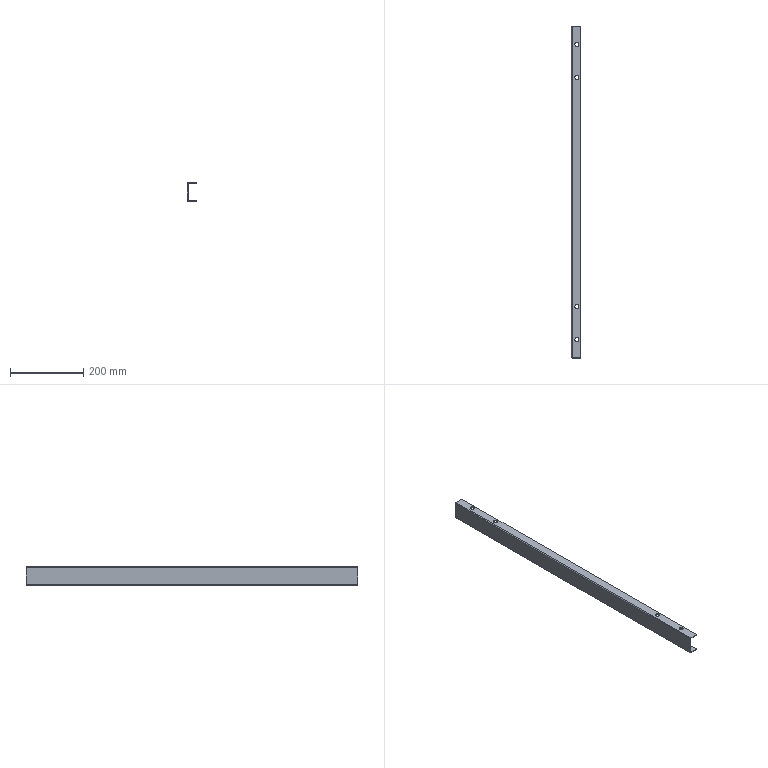Part | SolidWorks | features FlatPattern 1, ICE 1, SMBaseFlange 1, SheetMetal 1 | 1 solid | 38 faces | box 25 x 905 x 50 mm | volume 170375 mm3 | cylinder 20 | plane 18 | commonest cylinder face diameters 11 x16 0.4 x2 4.4 x2
STEP:
#1=CARTESIAN_POINT('',(20.5,402.5,-23.));
#2=VERTEX_POINT('',#1);
#3=CARTESIAN_POINT('',(9.5,402.5,-23.));
#4=VERTEX_POINT('',#3);
#5=CARTESIAN_POINT('',(15.,402.5,-23.));
#6=DIRECTION('',(0.,0.,-1.));
#7=DIRECTION('',(-1.,0.,0.));
#8=AXIS2_PLACEMENT_3D('',#5,#6,#7);
#9=CIRCLE('',#8,5.5);
#10=EDGE_CURVE('',#2,#4,#9,.T.);
#11=ORIENTED_EDGE('',*,*,#10,.F.);
#12=CARTESIAN_POINT('',(20.5,402.5,-25.));
#13=VERTEX_POINT('',#12);
#14=CARTESIAN_POINT('',(20.5,402.5,25.));
#15=DIRECTION('',(0.,0.,-1.));
#16=VECTOR('',#15,1000.);
#17=LINE('',#14,#16);
#18=EDGE_CURVE('',#2,#13,#17,.T.);
#19=ORIENTED_EDGE('',*,*,#18,.T.);
#20=CARTESIAN_POINT('',(9.5,402.5,-25.));
#21=VERTEX_POINT('',#20);
#22=CARTESIAN_POINT('',(15.,402.5,-25.));
#23=DIRECTION('',(0.,0.,-1.));
#24=DIRECTION('',(-1.,0.,0.));
#25=AXIS2_PLACEMENT_3D('',#22,#23,#24);
#26=CIRCLE('',#25,5.5);
#27=EDGE_CURVE('',#13,#21,#26,.T.);
#28=ORIENTED_EDGE('',*,*,#27,.T.);
#29=CARTESIAN_POINT('',(9.5,402.5,25.));
#30=DIRECTION('',(0.,0.,-1.));
#31=VECTOR('',#30,1000.);
#32=LINE('',#29,#31);
#33=EDGE_CURVE('',#4,#21,#32,.T.);
#34=ORIENTED_EDGE('',*,*,#33,.F.);
#35=EDGE_LOOP('',(#11,#19,#28,#34));
#36=FACE_OUTER_BOUND('',#35,.T.);
#37=CARTESIAN_POINT('',(15.,402.5,25.));
#38=DIRECTION('',(0.,0.,-1.));
#39=DIRECTION('',(-1.,0.,0.));
#40=AXIS2_PLACEMENT_3D('',#37,#38,#39);
#41=CYLINDRICAL_SURFACE('',#40,5.5);
#42=ADVANCED_FACE('',(#36),#41,.F.);
#43=CARTESIAN_POINT('',(20.5,312.5,-23.));
#44=VERTEX_POINT('',#43);
#45=CARTESIAN_POINT('',(9.5,312.5,-23.));
#46=VERTEX_POINT('',#45);
#47=CARTESIAN_POINT('',(15.,312.5,-23.));
#48=DIRECTION('',(0.,0.,-1.));
#49=DIRECTION('',(-1.,0.,0.));
#50=AXIS2_PLACEMENT_3D('',#47,#48,#49);
#51=CIRCLE('',#50,5.5);
#52=EDGE_CURVE('',#44,#46,#51,.T.);
#53=ORIENTED_EDGE('',*,*,#52,.F.);
#54=CARTESIAN_POINT('',(20.5,312.5,-25.));
#55=VERTEX_POINT('',#54);
#56=CARTESIAN_POINT('',(20.5,312.5,25.));
#57=DIRECTION('',(0.,0.,-1.));
#58=VECTOR('',#57,1000.);
#59=LINE('',#56,#58);
#60=EDGE_CURVE('',#44,#55,#59,.T.);
#61=ORIENTED_EDGE('',*,*,#60,.T.);
#62=CARTESIAN_POINT('',(9.5,312.5,-25.));
#63=VERTEX_POINT('',#62);
#64=CARTESIAN_POINT('',(15.,312.5,-25.));
#65=DIRECTION('',(0.,0.,-1.));
#66=DIRECTION('',(-1.,0.,0.));
#67=AXIS2_PLACEMENT_3D('',#64,#65,#66);
#68=CIRCLE('',#67,5.5);
#69=EDGE_CURVE('',#55,#63,#68,.T.);
#70=ORIENTED_EDGE('',*,*,#69,.T.);
#71=CARTESIAN_POINT('',(9.5,312.5,25.));
#72=DIRECTION('',(0.,0.,-1.));
#73=VECTOR('',#72,1000.);
#74=LINE('',#71,#73);
#75=EDGE_CURVE('',#46,#63,#74,.T.);
#76=ORIENTED_EDGE('',*,*,#75,.F.);
#77=EDGE_LOOP('',(#53,#61,#70,#76));
#78=FACE_OUTER_BOUND('',#77,.T.);
#79=CARTESIAN_POINT('',(15.,312.5,25.));
#80=DIRECTION('',(0.,0.,-1.));
#81=DIRECTION('',(-1.,0.,0.));
#82=AXIS2_PLACEMENT_3D('',#79,#80,#81);
#83=CYLINDRICAL_SURFACE('',#82,5.5);
#84=ADVANCED_FACE('',(#78),#83,.F.);
#85=CARTESIAN_POINT('',(20.5,-312.5,-23.));
#86=VERTEX_POINT('',#85);
#87=CARTESIAN_POINT('',(9.5,-312.5,-23.));
#88=VERTEX_POINT('',#87);
#89=CARTESIAN_POINT('',(15.,-312.5,-23.));
#90=DIRECTION('',(0.,0.,-1.));
#91=DIRECTION('',(-1.,0.,0.));
#92=AXIS2_PLACEMENT_3D('',#89,#90,#91);
#93=CIRCLE('',#92,5.5);
#94=EDGE_CURVE('',#86,#88,#93,.T.);
#95=ORIENTED_EDGE('',*,*,#94,.F.);
#96=CARTESIAN_POINT('',(20.5,-312.5,-25.));
#97=VERTEX_POINT('',#96);
#98=CARTESIAN_POINT('',(20.5,-312.5,25.));
#99=DIRECTION('',(0.,0.,-1.));
#100=VECTOR('',#99,1000.);
#101=LINE('',#98,#100);
#102=EDGE_CURVE('',#86,#97,#101,.T.);
#103=ORIENTED_EDGE('',*,*,#102,.T.);
#104=CARTESIAN_POINT('',(9.5,-312.5,-25.));
#105=VERTEX_POINT('',#104);
#106=CARTESIAN_POINT('',(15.,-312.5,-25.));
#107=DIRECTION('',(0.,0.,-1.));
#108=DIRECTION('',(-1.,0.,0.));
#109=AXIS2_PLACEMENT_3D('',#106,#107,#108);
#110=CIRCLE('',#109,5.5);
#111=EDGE_CURVE('',#97,#105,#110,.T.);
#112=ORIENTED_EDGE('',*,*,#111,.T.);
#113=CARTESIAN_POINT('',(9.5,-312.5,25.));
#114=DIRECTION('',(0.,0.,-1.));
#115=VECTOR('',#114,1000.);
#116=LINE('',#113,#115);
#117=EDGE_CURVE('',#88,#105,#116,.T.);
#118=ORIENTED_EDGE('',*,*,#117,.F.);
#119=EDGE_LOOP('',(#95,#103,#112,#118));
#120=FACE_OUTER_BOUND('',#119,.T.);
#121=CARTESIAN_POINT('',(15.,-312.5,25.));
#122=DIRECTION('',(0.,0.,-1.));
#123=DIRECTION('',(-1.,0.,0.));
#124=AXIS2_PLACEMENT_3D('',#121,#122,#123);
#125=CYLINDRICAL_SURFACE('',#124,5.5);
#126=ADVANCED_FACE('',(#120),#125,.F.);
#127=CARTESIAN_POINT('',(20.5,-402.5,-23.));
#128=VERTEX_POINT('',#127);
#129=CARTESIAN_POINT('',(9.5,-402.5,-23.));
#130=VERTEX_POINT('',#129);
#131=CARTESIAN_POINT('',(15.,-402.5,-23.));
#132=DIRECTION('',(0.,0.,-1.));
#133=DIRECTION('',(-1.,0.,0.));
#134=AXIS2_PLACEMENT_3D('',#131,#132,#133);
#135=CIRCLE('',#134,5.5);
#136=EDGE_CURVE('',#128,#130,#135,.T.);
#137=ORIENTED_EDGE('',*,*,#136,.F.);
#138=CARTESIAN_POINT('',(20.5,-402.5,-25.));
#139=VERTEX_POINT('',#138);
#140=CARTESIAN_POINT('',(20.5,-402.5,25.));
#141=DIRECTION('',(0.,0.,-1.));
#142=VECTOR('',#141,1000.);
#143=LINE('',#140,#142);
#144=EDGE_CURVE('',#128,#139,#143,.T.);
#145=ORIENTED_EDGE('',*,*,#144,.T.);
#146=CARTESIAN_POINT('',(9.5,-402.5,-25.));
#147=VERTEX_POINT('',#146);
#148=CARTESIAN_POINT('',(15.,-402.5,-25.));
#149=DIRECTION('',(0.,0.,-1.));
#150=DIRECTION('',(-1.,0.,0.));
#151=AXIS2_PLACEMENT_3D('',#148,#149,#150);
#152=CIRCLE('',#151,5.5);
#153=EDGE_CURVE('',#139,#147,#152,.T.);
#154=ORIENTED_EDGE('',*,*,#153,.T.);
#155=CARTESIAN_POINT('',(9.5,-402.5,25.));
#156=DIRECTION('',(0.,0.,-1.));
#157=VECTOR('',#156,1000.);
#158=LINE('',#155,#157);
#159=EDGE_CURVE('',#130,#147,#158,.T.);
#160=ORIENTED_EDGE('',*,*,#159,.F.);
#161=EDGE_LOOP('',(#137,#145,#154,#160));
#162=FACE_OUTER_BOUND('',#161,.T.);
#163=CARTESIAN_POINT('',(15.,-402.5,25.));
#164=DIRECTION('',(0.,0.,-1.));
#165=DIRECTION('',(-1.,0.,0.));
#166=AXIS2_PLACEMENT_3D('',#163,#164,#165);
#167=CYLINDRICAL_SURFACE('',#166,5.5);
#168=ADVANCED_FACE('',(#162),#167,.F.);
#169=CARTESIAN_POINT('',(20.5,402.5,25.));
#170=VERTEX_POINT('',#169);
#171=CARTESIAN_POINT('',(9.5,402.5,25.));
#172=VERTEX_POINT('',#171);
#173=CARTESIAN_POINT('',(15.,402.5,25.));
#174=DIRECTION('',(0.,0.,-1.));
#175=DIRECTION('',(-1.,0.,0.));
#176=AXIS2_PLACEMENT_3D('',#173,#174,#175);
#177=CIRCLE('',#176,5.5);
#178=EDGE_CURVE('',#170,#172,#177,.T.);
#179=ORIENTED_EDGE('',*,*,#178,.F.);
#180=CARTESIAN_POINT('',(20.5,402.5,23.));
#181=VERTEX_POINT('',#180);
#182=CARTESIAN_POINT('',(20.5,402.5,25.));
#183=DIRECTION('',(0.,0.,-1.));
#184=VECTOR('',#183,1000.);
#185=LINE('',#182,#184);
#186=EDGE_CURVE('',#170,#181,#185,.T.);
#187=ORIENTED_EDGE('',*,*,#186,.T.);
#188=CARTESIAN_POINT('',(9.5,402.5,23.));
#189=VERTEX_POINT('',#188);
#190=CARTESIAN_POINT('',(15.,402.5,23.));
#191=DIRECTION('',(0.,0.,1.));
#192=DIRECTION('',(1.,0.,0.));
#193=AXIS2_PLACEMENT_3D('',#190,#191,#192);
#194=CIRCLE('',#193,5.5);
#195=EDGE_CURVE('',#189,#181,#194,.T.);
#196=ORIENTED_EDGE('',*,*,#195,.F.);
#197=CARTESIAN_POINT('',(9.5,402.5,25.));
#198=DIRECTION('',(0.,0.,-1.));
#199=VECTOR('',#198,1000.);
#200=LINE('',#197,#199);
#201=EDGE_CURVE('',#172,#189,#200,.T.);
#202=ORIENTED_EDGE('',*,*,#201,.F.);
#203=EDGE_LOOP('',(#179,#187,#196,#202));
#204=FACE_OUTER_BOUND('',#203,.T.);
#205=CARTESIAN_POINT('',(15.,402.5,25.));
#206=DIRECTION('',(0.,0.,-1.));
#207=DIRECTION('',(-1.,0.,0.));
#208=AXIS2_PLACEMENT_3D('',#205,#206,#207);
#209=CYLINDRICAL_SURFACE('',#208,5.5);
#210=ADVANCED_FACE('',(#204),#209,.F.);
#211=CARTESIAN_POINT('',(20.5,312.5,25.));
#212=VERTEX_POINT('',#211);
#213=CARTESIAN_POINT('',(9.5,312.5,25.));
#214=VERTEX_POINT('',#213);
#215=CARTESIAN_POINT('',(15.,312.5,25.));
#216=DIRECTION('',(0.,0.,-1.));
#217=DIRECTION('',(-1.,0.,0.));
#218=AXIS2_PLACEMENT_3D('',#215,#216,#217);
#219=CIRCLE('',#218,5.5);
#220=EDGE_CURVE('',#212,#214,#219,.T.);
#221=ORIENTED_EDGE('',*,*,#220,.F.);
#222=CARTESIAN_POINT('',(20.5,312.5,23.));
#223=VERTEX_POINT('',#222);
#224=CARTESIAN_POINT('',(20.5,312.5,25.));
#225=DIRECTION('',(0.,0.,-1.));
#226=VECTOR('',#225,1000.);
#227=LINE('',#224,#226);
#228=EDGE_CURVE('',#212,#223,#227,.T.);
#229=ORIENTED_EDGE('',*,*,#228,.T.);
#230=CARTESIAN_POINT('',(9.5,312.5,23.));
#231=VERTEX_POINT('',#230);
#232=CARTESIAN_POINT('',(15.,312.5,23.));
#233=DIRECTION('',(0.,0.,1.));
#234=DIRECTION('',(1.,0.,0.));
#235=AXIS2_PLACEMENT_3D('',#232,#233,#234);
#236=CIRCLE('',#235,5.5);
#237=EDGE_CURVE('',#231,#223,#236,.T.);
#238=ORIENTED_EDGE('',*,*,#237,.F.);
#239=CARTESIAN_POINT('',(9.5,312.5,25.));
#240=DIRECTION('',(0.,0.,-1.));
#241=VECTOR('',#240,1000.);
#242=LINE('',#239,#241);
#243=EDGE_CURVE('',#214,#231,#242,.T.);
#244=ORIENTED_EDGE('',*,*,#243,.F.);
#245=EDGE_LOOP('',(#221,#229,#238,#244));
#246=FACE_OUTER_BOUND('',#245,.T.);
#247=CARTESIAN_POINT('',(15.,312.5,25.));
#248=DIRECTION('',(0.,0.,-1.));
#249=DIRECTION('',(-1.,0.,0.));
#250=AXIS2_PLACEMENT_3D('',#247,#248,#249);
#251=CYLINDRICAL_SURFACE('',#250,5.5);
#252=ADVANCED_FACE('',(#246),#251,.F.);
#253=CARTESIAN_POINT('',(20.5,-312.5,25.));
#254=VERTEX_POINT('',#253);
#255=CARTESIAN_POINT('',(9.5,-312.5,25.));
#256=VERTEX_POINT('',#255);
#257=CARTESIAN_POINT('',(15.,-312.5,25.));
#258=DIRECTION('',(0.,0.,-1.));
#259=DIRECTION('',(1.,0.,0.));
#260=AXIS2_PLACEMENT_3D('',#257,#258,#259);
#261=CIRCLE('',#260,5.5);
#262=EDGE_CURVE('',#254,#256,#261,.T.);
#263=ORIENTED_EDGE('',*,*,#262,.F.);
#264=CARTESIAN_POINT('',(20.5,-312.5,23.));
#265=VERTEX_POINT('',#264);
#266=CARTESIAN_POINT('',(20.5,-312.5,25.));
#267=DIRECTION('',(0.,0.,-1.));
#268=VECTOR('',#267,1000.);
#269=LINE('',#266,#268);
#270=EDGE_CURVE('',#254,#265,#269,.T.);
#271=ORIENTED_EDGE('',*,*,#270,.T.);
#272=CARTESIAN_POINT('',(9.5,-312.5,23.));
#273=VERTEX_POINT('',#272);
#274=CARTESIAN_POINT('',(15.,-312.5,23.));
#275=DIRECTION('',(0.,0.,1.));
#276=DIRECTION('',(1.,0.,0.));
#277=AXIS2_PLACEMENT_3D('',#274,#275,#276);
#278=CIRCLE('',#277,5.5);
#279=EDGE_CURVE('',#273,#265,#278,.T.);
#280=ORIENTED_EDGE('',*,*,#279,.F.);
#281=CARTESIAN_POINT('',(9.5,-312.5,25.));
#282=DIRECTION('',(0.,0.,-1.));
#283=VECTOR('',#282,1000.);
#284=LINE('',#281,#283);
#285=EDGE_CURVE('',#256,#273,#284,.T.);
#286=ORIENTED_EDGE('',*,*,#285,.F.);
#287=EDGE_LOOP('',(#263,#271,#280,#286));
#288=FACE_OUTER_BOUND('',#287,.T.);
#289=CARTESIAN_POINT('',(15.,-312.5,25.));
#290=DIRECTION('',(0.,0.,-1.));
#291=DIRECTION('',(-1.,0.,0.));
#292=AXIS2_PLACEMENT_3D('',#289,#290,#291);
#293=CYLINDRICAL_SURFACE('',#292,5.5);
#294=ADVANCED_FACE('',(#288),#293,.F.);
#295=CARTESIAN_POINT('',(20.5,-402.5,25.));
#296=VERTEX_POINT('',#295);
#297=CARTESIAN_POINT('',(9.5,-402.5,25.));
#298=VERTEX_POINT('',#297);
#299=CARTESIAN_POINT('',(15.,-402.5,25.));
#300=DIRECTION('',(0.,0.,-1.));
#301=DIRECTION('',(1.,0.,0.));
#302=AXIS2_PLACEMENT_3D('',#299,#300,#301);
#303=CIRCLE('',#302,5.5);
#304=EDGE_CURVE('',#296,#298,#303,.T.);
#305=ORIENTED_EDGE('',*,*,#304,.F.);
#306=CARTESIAN_POINT('',(20.5,-402.5,23.));
#307=VERTEX_POINT('',#306);
#308=CARTESIAN_POINT('',(20.5,-402.5,25.));
#309=DIRECTION('',(0.,0.,-1.));
#310=VECTOR('',#309,1000.);
#311=LINE('',#308,#310);
#312=EDGE_CURVE('',#296,#307,#311,.T.);
#313=ORIENTED_EDGE('',*,*,#312,.T.);
#314=CARTESIAN_POINT('',(9.5,-402.5,23.));
#315=VERTEX_POINT('',#314);
#316=CARTESIAN_POINT('',(15.,-402.5,23.));
#317=DIRECTION('',(0.,0.,1.));
#318=DIRECTION('',(1.,0.,0.));
#319=AXIS2_PLACEMENT_3D('',#316,#317,#318);
#320=CIRCLE('',#319,5.5);
#321=EDGE_CURVE('',#315,#307,#320,.T.);
#322=ORIENTED_EDGE('',*,*,#321,.F.);
#323=CARTESIAN_POINT('',(9.5,-402.5,25.));
#324=DIRECTION('',(0.,0.,-1.));
#325=VECTOR('',#324,1000.);
#326=LINE('',#323,#325);
#327=EDGE_CURVE('',#298,#315,#326,.T.);
#328=ORIENTED_EDGE('',*,*,#327,.F.);
#329=EDGE_LOOP('',(#305,#313,#322,#328));
#330=FACE_OUTER_BOUND('',#329,.T.);
#331=CARTESIAN_POINT('',(15.,-402.5,25.));
#332=DIRECTION('',(0.,0.,-1.));
#333=DIRECTION('',(-1.,0.,0.));
#334=AXIS2_PLACEMENT_3D('',#331,#332,#333);
#335=CYLINDRICAL_SURFACE('',#334,5.5);
#336=ADVANCED_FACE('',(#330),#335,.F.);
#337=CARTESIAN_POINT('',(0.,452.5,22.8));
#338=VERTEX_POINT('',#337);
#339=CARTESIAN_POINT('',(2.,452.5,22.8));
#340=VERTEX_POINT('',#339);
#341=CARTESIAN_POINT('',(0.,452.5,22.8));
#342=DIRECTION('',(1.,0.,0.));
#343=VECTOR('',#342,1000.);
#344=LINE('',#341,#343);
#345=EDGE_CURVE('',#338,#340,#344,.T.);
#346=ORIENTED_EDGE('',*,*,#345,.F.);
#347=CARTESIAN_POINT('',(2.2,452.5,25.));
#348=VERTEX_POINT('',#347);
#349=CARTESIAN_POINT('',(2.2,452.5,22.8));
#350=DIRECTION('',(0.,-1.,0.));
#351=DIRECTION('',(0.,0.,1.));
#352=AXIS2_PLACEMENT_3D('',#349,#350,#351);
#353=CIRCLE('',#352,2.2);
#354=EDGE_CURVE('',#348,#338,#353,.T.);
#355=ORIENTED_EDGE('',*,*,#354,.F.);
#356=CARTESIAN_POINT('',(2.2,452.5,23.));
#357=VERTEX_POINT('',#356);
#358=CARTESIAN_POINT('',(2.2,452.5,23.));
#359=DIRECTION('',(0.,0.,1.));
#360=VECTOR('',#359,1000.);
#361=LINE('',#358,#360);
#362=EDGE_CURVE('',#357,#348,#361,.T.);
#363=ORIENTED_EDGE('',*,*,#362,.F.);
#364=CARTESIAN_POINT('',(2.2,452.5,22.8));
#365=DIRECTION('',(0.,-1.,0.));
#366=DIRECTION('',(1.,0.,0.));
#367=AXIS2_PLACEMENT_3D('',#364,#365,#366);
#368=CIRCLE('',#367,0.2);
#369=EDGE_CURVE('',#357,#340,#368,.T.);
#370=ORIENTED_EDGE('',*,*,#369,.T.);
#371=EDGE_LOOP('',(#346,#355,#363,#370));
#372=FACE_OUTER_BOUND('',#371,.T.);
#373=CARTESIAN_POINT('',(0.,452.5,22.8));
#374=DIRECTION('',(0.,1.,0.));
#375=DIRECTION('',(0.,0.,1.));
#376=AXIS2_PLACEMENT_3D('',#373,#374,#375);
#377=PLANE('',#376);
#378=ADVANCED_FACE('',(#372),#377,.T.);
#379=CARTESIAN_POINT('',(0.,452.5,-22.8));
#380=VERTEX_POINT('',#379);
#381=CARTESIAN_POINT('',(0.,452.5,-25.));
#382=DIRECTION('',(0.,0.,-1.));
#383=VECTOR('',#382,1000.);
#384=LINE('',#381,#383);
#385=EDGE_CURVE('',#338,#380,#384,.T.);
#386=ORIENTED_EDGE('',*,*,#385,.F.);
#387=ORIENTED_EDGE('',*,*,#345,.T.);
#388=CARTESIAN_POINT('',(2.,452.5,-22.8));
#389=VERTEX_POINT('',#388);
#390=CARTESIAN_POINT('',(2.,452.5,-25.));
#391=DIRECTION('',(0.,0.,-1.));
#392=VECTOR('',#391,1000.);
#393=LINE('',#390,#392);
#394=EDGE_CURVE('',#340,#389,#393,.T.);
#395=ORIENTED_EDGE('',*,*,#394,.T.);
#396=CARTESIAN_POINT('',(2.,452.5,-22.8));
#397=DIRECTION('',(-1.,0.,0.));
#398=VECTOR('',#397,1000.);
#399=LINE('',#396,#398);
#400=EDGE_CURVE('',#389,#380,#399,.T.);
#401=ORIENTED_EDGE('',*,*,#400,.T.);
#402=EDGE_LOOP('',(#386,#387,#395,#401));
#403=FACE_OUTER_BOUND('',#402,.T.);
#404=CARTESIAN_POINT('',(2.2,452.5,23.));
#405=DIRECTION('',(0.,1.,0.));
#406=DIRECTION('',(0.,0.,1.));
#407=AXIS2_PLACEMENT_3D('',#404,#405,#406);
#408=PLANE('',#407);
#409=ADVANCED_FACE('',(#403),#408,.T.);
#410=CARTESIAN_POINT('',(2.2,-452.5,25.));
#411=VERTEX_POINT('',#410);
#412=CARTESIAN_POINT('',(2.2,-452.5,23.));
#413=VERTEX_POINT('',#412);
#414=CARTESIAN_POINT('',(2.2,-452.5,25.));
#415=DIRECTION('',(0.,0.,-1.));
#416=VECTOR('',#415,1000.);
#417=LINE('',#414,#416);
#418=EDGE_CURVE('',#411,#413,#417,.T.);
#419=ORIENTED_EDGE('',*,*,#418,.F.);
#420=CARTESIAN_POINT('',(0.,-452.5,22.8));
#421=VERTEX_POINT('',#420);
#422=CARTESIAN_POINT('',(2.2,-452.5,22.8));
#423=DIRECTION('',(0.,-1.,0.));
#424=DIRECTION('',(0.,0.,1.));
#425=AXIS2_PLACEMENT_3D('',#422,#423,#424);
#426=CIRCLE('',#425,2.2);
#427=EDGE_CURVE('',#411,#421,#426,.T.);
#428=ORIENTED_EDGE('',*,*,#427,.T.);
#429=CARTESIAN_POINT('',(2.,-452.5,22.8));
#430=VERTEX_POINT('',#429);
#431=CARTESIAN_POINT('',(2.,-452.5,22.8));
#432=DIRECTION('',(-1.,0.,0.));
#433=VECTOR('',#432,1000.);
#434=LINE('',#431,#433);
#435=EDGE_CURVE('',#430,#421,#434,.T.);
#436=ORIENTED_EDGE('',*,*,#435,.F.);
#437=CARTESIAN_POINT('',(2.2,-452.5,22.8));
#438=DIRECTION('',(0.,-1.,0.));
#439=DIRECTION('',(1.,0.,0.));
#440=AXIS2_PLACEMENT_3D('',#437,#438,#439);
#441=CIRCLE('',#440,0.2);
#442=EDGE_CURVE('',#413,#430,#441,.T.);
#443=ORIENTED_EDGE('',*,*,#442,.F.);
#444=EDGE_LOOP('',(#419,#428,#436,#443));
#445=FACE_OUTER_BOUND('',#444,.T.);
#446=CARTESIAN_POINT('',(2.2,-452.5,25.));
#447=DIRECTION('',(0.,-1.,0.));
#448=DIRECTION('',(0.,0.,-1.));
#449=AXIS2_PLACEMENT_3D('',#446,#447,#448);
#450=PLANE('',#449);
#451=ADVANCED_FACE('',(#445),#450,.T.);
#452=CARTESIAN_POINT('',(25.,-452.5,25.));
#453=VERTEX_POINT('',#452);
#454=CARTESIAN_POINT('',(0.,-452.5,25.));
#455=DIRECTION('',(-1.,0.,0.));
#456=VECTOR('',#455,1000.);
#457=LINE('',#454,#456);
#458=EDGE_CURVE('',#453,#411,#457,.T.);
#459=ORIENTED_EDGE('',*,*,#458,.T.);
#460=ORIENTED_EDGE('',*,*,#418,.T.);
#461=CARTESIAN_POINT('',(25.,-452.5,23.));
#462=VERTEX_POINT('',#461);
#463=CARTESIAN_POINT('',(0.,-452.5,23.));
#464=DIRECTION('',(-1.,0.,0.));
#465=VECTOR('',#464,1000.);
#466=LINE('',#463,#465);
#467=EDGE_CURVE('',#462,#413,#466,.T.);
#468=ORIENTED_EDGE('',*,*,#467,.F.);
#469=CARTESIAN_POINT('',(25.,-452.5,23.));
#470=DIRECTION('',(0.,0.,1.));
#471=VECTOR('',#470,1000.);
#472=LINE('',#469,#471);
#473=EDGE_CURVE('',#462,#453,#472,.T.);
#474=ORIENTED_EDGE('',*,*,#473,.T.);
#475=EDGE_LOOP('',(#459,#460,#468,#474));
#476=FACE_OUTER_BOUND('',#475,.T.);
#477=CARTESIAN_POINT('',(2.,-452.5,22.8));
#478=DIRECTION('',(0.,-1.,0.));
#479=DIRECTION('',(0.,0.,-1.));
#480=AXIS2_PLACEMENT_3D('',#477,#478,#479);
#481=PLANE('',#480);
#482=ADVANCED_FACE('',(#476),#481,.T.);
#483=CARTESIAN_POINT('',(2.2,452.5,-25.));
#484=VERTEX_POINT('',#483);
#485=CARTESIAN_POINT('',(2.2,452.5,-23.));
#486=VERTEX_POINT('',#485);
#487=CARTESIAN_POINT('',(2.2,452.5,-25.));
#488=DIRECTION('',(0.,0.,1.));
#489=VECTOR('',#488,1000.);
#490=LINE('',#487,#489);
#491=EDGE_CURVE('',#484,#486,#490,.T.);
#492=ORIENTED_EDGE('',*,*,#491,.F.);
#493=CARTESIAN_POINT('',(2.2,452.5,-22.8));
#494=DIRECTION('',(0.,-1.,0.));
#495=DIRECTION('',(0.,0.,1.));
#496=AXIS2_PLACEMENT_3D('',#493,#494,#495);
#497=CIRCLE('',#496,2.2);
#498=EDGE_CURVE('',#380,#484,#497,.T.);
#499=ORIENTED_EDGE('',*,*,#498,.F.);
#500=ORIENTED_EDGE('',*,*,#400,.F.);
#501=CARTESIAN_POINT('',(2.2,452.5,-22.8));
#502=DIRECTION('',(0.,-1.,0.));
#503=DIRECTION('',(1.,0.,0.));
#504=AXIS2_PLACEMENT_3D('',#501,#502,#503);
#505=CIRCLE('',#504,0.2);
#506=EDGE_CURVE('',#389,#486,#505,.T.);
#507=ORIENTED_EDGE('',*,*,#506,.T.);
#508=EDGE_LOOP('',(#492,#499,#500,#507));
#509=FACE_OUTER_BOUND('',#508,.T.);
#510=CARTESIAN_POINT('',(2.2,452.5,-25.));
#511=DIRECTION('',(0.,1.,0.));
#512=DIRECTION('',(0.,0.,1.));
#513=AXIS2_PLACEMENT_3D('',#510,#511,#512);
#514=PLANE('',#513);
#515=ADVANCED_FACE('',(#509),#514,.T.);
#516=CARTESIAN_POINT('',(25.,452.5,-25.));
#517=VERTEX_POINT('',#516);
#518=CARTESIAN_POINT('',(0.,452.5,-25.));
#519=DIRECTION('',(1.,0.,0.));
#520=VECTOR('',#519,1000.);
#521=LINE('',#518,#520);
#522=EDGE_CURVE('',#484,#517,#521,.T.);
#523=ORIENTED_EDGE('',*,*,#522,.F.);
#524=ORIENTED_EDGE('',*,*,#491,.T.);
#525=CARTESIAN_POINT('',(25.,452.5,-23.));
#526=VERTEX_POINT('',#525);
#527=CARTESIAN_POINT('',(0.,452.5,-23.));
#528=DIRECTION('',(1.,0.,0.));
#529=VECTOR('',#528,1000.);
#530=LINE('',#527,#529);
#531=EDGE_CURVE('',#486,#526,#530,.T.);
#532=ORIENTED_EDGE('',*,*,#531,.T.);
#533=CARTESIAN_POINT('',(25.,452.5,-25.));
#534=DIRECTION('',(0.,0.,1.));
#535=VECTOR('',#534,1000.);
#536=LINE('',#533,#535);
#537=EDGE_CURVE('',#517,#526,#536,.T.);
#538=ORIENTED_EDGE('',*,*,#537,.F.);
#539=EDGE_LOOP('',(#523,#524,#532,#538));
#540=FACE_OUTER_BOUND('',#539,.T.);
#541=CARTESIAN_POINT('',(2.,452.5,-22.8));
#542=DIRECTION('',(0.,1.,0.));
#543=DIRECTION('',(0.,0.,1.));
#544=AXIS2_PLACEMENT_3D('',#541,#542,#543);
#545=PLANE('',#544);
#546=ADVANCED_FACE('',(#540),#545,.T.);
#547=CARTESIAN_POINT('',(0.,-452.5,-22.8));
#548=VERTEX_POINT('',#547);
#549=CARTESIAN_POINT('',(2.,-452.5,-22.8));
#550=VERTEX_POINT('',#549);
#551=CARTESIAN_POINT('',(0.,-452.5,-22.8));
#552=DIRECTION('',(1.,0.,0.));
#553=VECTOR('',#552,1000.);
#554=LINE('',#551,#553);
#555=EDGE_CURVE('',#548,#550,#554,.T.);
#556=ORIENTED_EDGE('',*,*,#555,.F.);
#557=CARTESIAN_POINT('',(2.2,-452.5,-25.));
#558=VERTEX_POINT('',#557);
#559=CARTESIAN_POINT('',(2.2,-452.5,-22.8));
#560=DIRECTION('',(0.,-1.,0.));
#561=DIRECTION('',(0.,0.,1.));
#562=AXIS2_PLACEMENT_3D('',#559,#560,#561);
#563=CIRCLE('',#562,2.2);
#564=EDGE_CURVE('',#548,#558,#563,.T.);
#565=ORIENTED_EDGE('',*,*,#564,.T.);
#566=CARTESIAN_POINT('',(2.2,-452.5,-23.));
#567=VERTEX_POINT('',#566);
#568=CARTESIAN_POINT('',(2.2,-452.5,-23.));
#569=DIRECTION('',(0.,0.,-1.));
#570=VECTOR('',#569,1000.);
#571=LINE('',#568,#570);
#572=EDGE_CURVE('',#567,#558,#571,.T.);
#573=ORIENTED_EDGE('',*,*,#572,.F.);
#574=CARTESIAN_POINT('',(2.2,-452.5,-22.8));
#575=DIRECTION('',(0.,-1.,0.));
#576=DIRECTION('',(1.,0.,0.));
#577=AXIS2_PLACEMENT_3D('',#574,#575,#576);
#578=CIRCLE('',#577,0.2);
#579=EDGE_CURVE('',#550,#567,#578,.T.);
#580=ORIENTED_EDGE('',*,*,#579,.F.);
#581=EDGE_LOOP('',(#556,#565,#573,#580));
#582=FACE_OUTER_BOUND('',#581,.T.);
#583=CARTESIAN_POINT('',(0.,-452.5,-22.8));
#584=DIRECTION('',(0.,-1.,0.));
#585=DIRECTION('',(0.,0.,-1.));
#586=AXIS2_PLACEMENT_3D('',#583,#584,#585);
#587=PLANE('',#586);
#588=ADVANCED_FACE('',(#582),#587,.T.);
#589=CARTESIAN_POINT('',(0.,-452.5,-25.));
#590=DIRECTION('',(0.,0.,-1.));
#591=VECTOR('',#590,1000.);
#592=LINE('',#589,#591);
#593=EDGE_CURVE('',#421,#548,#592,.T.);
#594=ORIENTED_EDGE('',*,*,#593,.T.);
#595=ORIENTED_EDGE('',*,*,#555,.T.);
#596=CARTESIAN_POINT('',(2.,-452.5,-25.));
#597=DIRECTION('',(0.,0.,-1.));
#598=VECTOR('',#597,1000.);
#599=LINE('',#596,#598);
#600=EDGE_CURVE('',#430,#550,#599,.T.);
#601=ORIENTED_EDGE('',*,*,#600,.F.);
#602=ORIENTED_EDGE('',*,*,#435,.T.);
#603=EDGE_LOOP('',(#594,#595,#601,#602));
#604=FACE_OUTER_BOUND('',#603,.T.);
#605=CARTESIAN_POINT('',(2.2,-452.5,-23.));
#606=DIRECTION('',(0.,-1.,0.));
#607=DIRECTION('',(0.,0.,-1.));
#608=AXIS2_PLACEMENT_3D('',#605,#606,#607);
#609=PLANE('',#608);
#610=ADVANCED_FACE('',(#604),#609,.T.);
#611=CARTESIAN_POINT('',(15.,402.5,-23.));
#612=DIRECTION('',(0.,0.,-1.));
#613=DIRECTION('',(-1.,0.,0.));
#614=AXIS2_PLACEMENT_3D('',#611,#612,#613);
#615=CIRCLE('',#614,5.5);
#616=EDGE_CURVE('',#4,#2,#615,.T.);
#617=ORIENTED_EDGE('',*,*,#616,.T.);
#618=ORIENTED_EDGE('',*,*,#10,.T.);
#619=EDGE_LOOP('',(#617,#618));
#620=FACE_BOUND('',#619,.T.);
#621=CARTESIAN_POINT('',(15.,312.5,-23.));
#622=DIRECTION('',(0.,0.,-1.));
#623=DIRECTION('',(-1.,0.,0.));
#624=AXIS2_PLACEMENT_3D('',#621,#622,#623);
#625=CIRCLE('',#624,5.5);
#626=EDGE_CURVE('',#46,#44,#625,.T.);
#627=ORIENTED_EDGE('',*,*,#626,.T.);
#628=ORIENTED_EDGE('',*,*,#52,.T.);
#629=EDGE_LOOP('',(#627,#628));
#630=FACE_BOUND('',#629,.T.);
#631=CARTESIAN_POINT('',(15.,-312.5,-23.));
#632=DIRECTION('',(0.,0.,-1.));
#633=DIRECTION('',(-1.,0.,0.));
#634=AXIS2_PLACEMENT_3D('',#631,#632,#633);
#635=CIRCLE('',#634,5.5);
#636=EDGE_CURVE('',#88,#86,#635,.T.);
#637=ORIENTED_EDGE('',*,*,#636,.T.);
#638=ORIENTED_EDGE('',*,*,#94,.T.);
#639=EDGE_LOOP('',(#637,#638));
#640=FACE_BOUND('',#639,.T.);
#641=CARTESIAN_POINT('',(15.,-402.5,-23.));
#642=DIRECTION('',(0.,0.,-1.));
#643=DIRECTION('',(-1.,0.,0.));
#644=AXIS2_PLACEMENT_3D('',#641,#642,#643);
#645=CIRCLE('',#644,5.5);
#646=EDGE_CURVE('',#130,#128,#645,.T.);
#647=ORIENTED_EDGE('',*,*,#646,.T.);
#648=ORIENTED_EDGE('',*,*,#136,.T.);
#649=EDGE_LOOP('',(#647,#648));
#650=FACE_BOUND('',#649,.T.);
#651=CARTESIAN_POINT('',(25.,-452.5,-23.));
#652=VERTEX_POINT('',#651);
#653=CARTESIAN_POINT('',(0.,-452.5,-23.));
#654=DIRECTION('',(1.,0.,0.));
#655=VECTOR('',#654,1000.);
#656=LINE('',#653,#655);
#657=EDGE_CURVE('',#567,#652,#656,.T.);
#658=ORIENTED_EDGE('',*,*,#657,.T.);
#659=CARTESIAN_POINT('',(25.,452.5,-23.));
#660=DIRECTION('',(0.,-1.,0.));
#661=VECTOR('',#660,1000.);
#662=LINE('',#659,#661);
#663=EDGE_CURVE('',#526,#652,#662,.T.);
#664=ORIENTED_EDGE('',*,*,#663,.F.);
#665=ORIENTED_EDGE('',*,*,#531,.F.);
#666=CARTESIAN_POINT('',(2.2,452.5,-23.));
#667=DIRECTION('',(0.,-1.,0.));
#668=VECTOR('',#667,1000.);
#669=LINE('',#666,#668);
#670=EDGE_CURVE('',#486,#567,#669,.T.);
#671=ORIENTED_EDGE('',*,*,#670,.T.);
#672=EDGE_LOOP('',(#658,#664,#665,#671));
#673=FACE_OUTER_BOUND('',#672,.T.);
#674=CARTESIAN_POINT('',(0.,452.5,-23.));
#675=DIRECTION('',(0.,0.,-1.));
#676=DIRECTION('',(-1.,0.,0.));
#677=AXIS2_PLACEMENT_3D('',#674,#675,#676);
#678=PLANE('',#677);
#679=ADVANCED_FACE('',(#620,#630,#640,#650,#673),#678,.F.);
#680=CARTESIAN_POINT('',(25.,-452.5,-25.));
#681=VERTEX_POINT('',#680);
#682=CARTESIAN_POINT('',(25.,-452.5,-25.));
#683=DIRECTION('',(0.,0.,1.));
#684=VECTOR('',#683,1000.);
#685=LINE('',#682,#684);
#686=EDGE_CURVE('',#681,#652,#685,.T.);
#687=ORIENTED_EDGE('',*,*,#686,.F.);
#688=CARTESIAN_POINT('',(25.,452.5,-25.));
#689=DIRECTION('',(0.,-1.,0.));
#690=VECTOR('',#689,1000.);
#691=LINE('',#688,#690);
#692=EDGE_CURVE('',#517,#681,#691,.T.);
#693=ORIENTED_EDGE('',*,*,#692,.F.);
#694=ORIENTED_EDGE('',*,*,#537,.T.);
#695=ORIENTED_EDGE('',*,*,#663,.T.);
#696=EDGE_LOOP('',(#687,#693,#694,#695));
#697=FACE_OUTER_BOUND('',#696,.T.);
#698=CARTESIAN_POINT('',(25.,452.5,-25.));
#699=DIRECTION('',(1.,0.,0.));
#700=DIRECTION('',(0.,0.,-1.));
#701=AXIS2_PLACEMENT_3D('',#698,#699,#700);
#702=PLANE('',#701);
#703=ADVANCED_FACE('',(#697),#702,.T.);
#704=CARTESIAN_POINT('',(15.,402.5,-25.));
#705=DIRECTION('',(0.,0.,-1.));
#706=DIRECTION('',(-1.,0.,0.));
#707=AXIS2_PLACEMENT_3D('',#704,#705,#706);
#708=CIRCLE('',#707,5.5);
#709=EDGE_CURVE('',#21,#13,#708,.T.);
#710=ORIENTED_EDGE('',*,*,#709,.F.);
#711=ORIENTED_EDGE('',*,*,#27,.F.);
#712=EDGE_LOOP('',(#710,#711));
#713=FACE_BOUND('',#712,.T.);
#714=CARTESIAN_POINT('',(15.,312.5,-25.));
#715=DIRECTION('',(0.,0.,-1.));
#716=DIRECTION('',(-1.,0.,0.));
#717=AXIS2_PLACEMENT_3D('',#714,#715,#716);
#718=CIRCLE('',#717,5.5);
#719=EDGE_CURVE('',#63,#55,#718,.T.);
#720=ORIENTED_EDGE('',*,*,#719,.F.);
#721=ORIENTED_EDGE('',*,*,#69,.F.);
#722=EDGE_LOOP('',(#720,#721));
#723=FACE_BOUND('',#722,.T.);
#724=CARTESIAN_POINT('',(15.,-312.5,-25.));
#725=DIRECTION('',(0.,0.,-1.));
#726=DIRECTION('',(-1.,0.,0.));
#727=AXIS2_PLACEMENT_3D('',#724,#725,#726);
#728=CIRCLE('',#727,5.5);
#729=EDGE_CURVE('',#105,#97,#728,.T.);
#730=ORIENTED_EDGE('',*,*,#729,.F.);
#731=ORIENTED_EDGE('',*,*,#111,.F.);
#732=EDGE_LOOP('',(#730,#731));
#733=FACE_BOUND('',#732,.T.);
#734=CARTESIAN_POINT('',(15.,-402.5,-25.));
#735=DIRECTION('',(0.,0.,-1.));
#736=DIRECTION('',(-1.,0.,0.));
#737=AXIS2_PLACEMENT_3D('',#734,#735,#736);
#738=CIRCLE('',#737,5.5);
#739=EDGE_CURVE('',#147,#139,#738,.T.);
#740=ORIENTED_EDGE('',*,*,#739,.F.);
#741=ORIENTED_EDGE('',*,*,#153,.F.);
#742=EDGE_LOOP('',(#740,#741));
#743=FACE_BOUND('',#742,.T.);
#744=CARTESIAN_POINT('',(0.,-452.5,-25.));
#745=DIRECTION('',(1.,0.,0.));
#746=VECTOR('',#745,1000.);
#747=LINE('',#744,#746);
#748=EDGE_CURVE('',#558,#681,#747,.T.);
#749=ORIENTED_EDGE('',*,*,#748,.F.);
#750=CARTESIAN_POINT('',(2.2,452.5,-25.));
#751=DIRECTION('',(0.,-1.,0.));
#752=VECTOR('',#751,1000.);
#753=LINE('',#750,#752);
#754=EDGE_CURVE('',#484,#558,#753,.T.);
#755=ORIENTED_EDGE('',*,*,#754,.F.);
#756=ORIENTED_EDGE('',*,*,#522,.T.);
#757=ORIENTED_EDGE('',*,*,#692,.T.);
#758=EDGE_LOOP('',(#749,#755,#756,#757));
#759=FACE_OUTER_BOUND('',#758,.T.);
#760=CARTESIAN_POINT('',(0.,452.5,-25.));
#761=DIRECTION('',(0.,0.,-1.));
#762=DIRECTION('',(-1.,0.,0.));
#763=AXIS2_PLACEMENT_3D('',#760,#761,#762);
#764=PLANE('',#763);
#765=ADVANCED_FACE('',(#713,#723,#733,#743,#759),#764,.T.);
#766=ORIENTED_EDGE('',*,*,#564,.F.);
#767=CARTESIAN_POINT('',(0.,452.5,-22.8));
#768=DIRECTION('',(0.,-1.,0.));
#769=VECTOR('',#768,1000.);
#770=LINE('',#767,#769);
#771=EDGE_CURVE('',#380,#548,#770,.T.);
#772=ORIENTED_EDGE('',*,*,#771,.F.);
#773=ORIENTED_EDGE('',*,*,#498,.T.);
#774=ORIENTED_EDGE('',*,*,#754,.T.);
#775=EDGE_LOOP('',(#766,#772,#773,#774));
#776=FACE_OUTER_BOUND('',#775,.T.);
#777=CARTESIAN_POINT('',(2.2,452.5,-22.8));
#778=DIRECTION('',(0.,-1.,0.));
#779=DIRECTION('',(0.,0.,-1.));
#780=AXIS2_PLACEMENT_3D('',#777,#778,#779);
#781=CYLINDRICAL_SURFACE('',#780,2.2);
#782=ADVANCED_FACE('',(#776),#781,.T.);
#783=ORIENTED_EDGE('',*,*,#593,.F.);
#784=CARTESIAN_POINT('',(0.,452.5,22.8));
#785=DIRECTION('',(0.,-1.,0.));
#786=VECTOR('',#785,1000.);
#787=LINE('',#784,#786);
#788=EDGE_CURVE('',#338,#421,#787,.T.);
#789=ORIENTED_EDGE('',*,*,#788,.F.);
#790=ORIENTED_EDGE('',*,*,#385,.T.);
#791=ORIENTED_EDGE('',*,*,#771,.T.);
#792=EDGE_LOOP('',(#783,#789,#790,#791));
#793=FACE_OUTER_BOUND('',#792,.T.);
#794=CARTESIAN_POINT('',(0.,452.5,-25.));
#795=DIRECTION('',(-1.,0.,0.));
#796=DIRECTION('',(0.,0.,1.));
#797=AXIS2_PLACEMENT_3D('',#794,#795,#796);
#798=PLANE('',#797);
#799=ADVANCED_FACE('',(#793),#798,.T.);
#800=ORIENTED_EDGE('',*,*,#427,.F.);
#801=CARTESIAN_POINT('',(2.2,452.5,25.));
#802=DIRECTION('',(0.,-1.,0.));
#803=VECTOR('',#802,1000.);
#804=LINE('',#801,#803);
#805=EDGE_CURVE('',#348,#411,#804,.T.);
#806=ORIENTED_EDGE('',*,*,#805,.F.);
#807=ORIENTED_EDGE('',*,*,#354,.T.);
#808=ORIENTED_EDGE('',*,*,#788,.T.);
#809=EDGE_LOOP('',(#800,#806,#807,#808));
#810=FACE_OUTER_BOUND('',#809,.T.);
#811=CARTESIAN_POINT('',(2.2,452.5,22.8));
#812=DIRECTION('',(0.,-1.,0.));
#813=DIRECTION('',(0.,0.,-1.));
#814=AXIS2_PLACEMENT_3D('',#811,#812,#813);
#815=CYLINDRICAL_SURFACE('',#814,2.2);
#816=ADVANCED_FACE('',(#810),#815,.T.);
#817=CARTESIAN_POINT('',(15.,402.5,25.));
#818=DIRECTION('',(0.,0.,-1.));
#819=DIRECTION('',(-1.,0.,0.));
#820=AXIS2_PLACEMENT_3D('',#817,#818,#819);
#821=CIRCLE('',#820,5.5);
#822=EDGE_CURVE('',#172,#170,#821,.T.);
#823=ORIENTED_EDGE('',*,*,#822,.T.);
#824=ORIENTED_EDGE('',*,*,#178,.T.);
#825=EDGE_LOOP('',(#823,#824));
#826=FACE_BOUND('',#825,.T.);
#827=CARTESIAN_POINT('',(15.,312.5,25.));
#828=DIRECTION('',(0.,0.,-1.));
#829=DIRECTION('',(-1.,0.,0.));
#830=AXIS2_PLACEMENT_3D('',#827,#828,#829);
#831=CIRCLE('',#830,5.5);
#832=EDGE_CURVE('',#214,#212,#831,.T.);
#833=ORIENTED_EDGE('',*,*,#832,.T.);
#834=ORIENTED_EDGE('',*,*,#220,.T.);
#835=EDGE_LOOP('',(#833,#834));
#836=FACE_BOUND('',#835,.T.);
#837=CARTESIAN_POINT('',(15.,-312.5,25.));
#838=DIRECTION('',(0.,0.,-1.));
#839=DIRECTION('',(1.,0.,0.));
#840=AXIS2_PLACEMENT_3D('',#837,#838,#839);
#841=CIRCLE('',#840,5.5);
#842=EDGE_CURVE('',#256,#254,#841,.T.);
#843=ORIENTED_EDGE('',*,*,#842,.T.);
#844=ORIENTED_EDGE('',*,*,#262,.T.);
#845=EDGE_LOOP('',(#843,#844));
#846=FACE_BOUND('',#845,.T.);
#847=CARTESIAN_POINT('',(15.,-402.5,25.));
#848=DIRECTION('',(0.,0.,-1.));
#849=DIRECTION('',(1.,0.,0.));
#850=AXIS2_PLACEMENT_3D('',#847,#848,#849);
#851=CIRCLE('',#850,5.5);
#852=EDGE_CURVE('',#298,#296,#851,.T.);
#853=ORIENTED_EDGE('',*,*,#852,.T.);
#854=ORIENTED_EDGE('',*,*,#304,.T.);
#855=EDGE_LOOP('',(#853,#854));
#856=FACE_BOUND('',#855,.T.);
#857=ORIENTED_EDGE('',*,*,#458,.F.);
#858=CARTESIAN_POINT('',(25.,452.5,25.));
#859=VERTEX_POINT('',#858);
#860=CARTESIAN_POINT('',(25.,452.5,25.));
#861=DIRECTION('',(0.,-1.,0.));
#862=VECTOR('',#861,1000.);
#863=LINE('',#860,#862);
#864=EDGE_CURVE('',#859,#453,#863,.T.);
#865=ORIENTED_EDGE('',*,*,#864,.F.);
#866=CARTESIAN_POINT('',(0.,452.5,25.));
#867=DIRECTION('',(-1.,0.,0.));
#868=VECTOR('',#867,1000.);
#869=LINE('',#866,#868);
#870=EDGE_CURVE('',#859,#348,#869,.T.);
#871=ORIENTED_EDGE('',*,*,#870,.T.);
#872=ORIENTED_EDGE('',*,*,#805,.T.);
#873=EDGE_LOOP('',(#857,#865,#871,#872));
#874=FACE_OUTER_BOUND('',#873,.T.);
#875=CARTESIAN_POINT('',(0.,452.5,25.));
#876=DIRECTION('',(0.,0.,1.));
#877=DIRECTION('',(1.,0.,0.));
#878=AXIS2_PLACEMENT_3D('',#875,#876,#877);
#879=PLANE('',#878);
#880=ADVANCED_FACE('',(#826,#836,#846,#856,#874),#879,.T.);
#881=ORIENTED_EDGE('',*,*,#473,.F.);
#882=CARTESIAN_POINT('',(25.,452.5,23.));
#883=VERTEX_POINT('',#882);
#884=CARTESIAN_POINT('',(25.,452.5,23.));
#885=DIRECTION('',(0.,-1.,0.));
#886=VECTOR('',#885,1000.);
#887=LINE('',#884,#886);
#888=EDGE_CURVE('',#883,#462,#887,.T.);
#889=ORIENTED_EDGE('',*,*,#888,.F.);
#890=CARTESIAN_POINT('',(25.,452.5,23.));
#891=DIRECTION('',(0.,0.,1.));
#892=VECTOR('',#891,1000.);
#893=LINE('',#890,#892);
#894=EDGE_CURVE('',#883,#859,#893,.T.);
#895=ORIENTED_EDGE('',*,*,#894,.T.);
#896=ORIENTED_EDGE('',*,*,#864,.T.);
#897=EDGE_LOOP('',(#881,#889,#895,#896));
#898=FACE_OUTER_BOUND('',#897,.T.);
#899=CARTESIAN_POINT('',(25.,452.5,23.));
#900=DIRECTION('',(1.,0.,0.));
#901=DIRECTION('',(0.,0.,-1.));
#902=AXIS2_PLACEMENT_3D('',#899,#900,#901);
#903=PLANE('',#902);
#904=ADVANCED_FACE('',(#898),#903,.T.);
#905=ORIENTED_EDGE('',*,*,#195,.T.);
#906=CARTESIAN_POINT('',(15.,402.5,23.));
#907=DIRECTION('',(0.,0.,1.));
#908=DIRECTION('',(1.,0.,0.));
#909=AXIS2_PLACEMENT_3D('',#906,#907,#908);
#910=CIRCLE('',#909,5.5);
#911=EDGE_CURVE('',#181,#189,#910,.T.);
#912=ORIENTED_EDGE('',*,*,#911,.T.);
#913=EDGE_LOOP('',(#905,#912));
#914=FACE_BOUND('',#913,.T.);
#915=ORIENTED_EDGE('',*,*,#237,.T.);
#916=CARTESIAN_POINT('',(15.,312.5,23.));
#917=DIRECTION('',(0.,0.,1.));
#918=DIRECTION('',(1.,0.,0.));
#919=AXIS2_PLACEMENT_3D('',#916,#917,#918);
#920=CIRCLE('',#919,5.5);
#921=EDGE_CURVE('',#223,#231,#920,.T.);
#922=ORIENTED_EDGE('',*,*,#921,.T.);
#923=EDGE_LOOP('',(#915,#922));
#924=FACE_BOUND('',#923,.T.);
#925=ORIENTED_EDGE('',*,*,#279,.T.);
#926=CARTESIAN_POINT('',(15.,-312.5,23.));
#927=DIRECTION('',(0.,0.,1.));
#928=DIRECTION('',(1.,0.,0.));
#929=AXIS2_PLACEMENT_3D('',#926,#927,#928);
#930=CIRCLE('',#929,5.5);
#931=EDGE_CURVE('',#265,#273,#930,.T.);
#932=ORIENTED_EDGE('',*,*,#931,.T.);
#933=EDGE_LOOP('',(#925,#932));
#934=FACE_BOUND('',#933,.T.);
#935=ORIENTED_EDGE('',*,*,#321,.T.);
#936=CARTESIAN_POINT('',(15.,-402.5,23.));
#937=DIRECTION('',(0.,0.,1.));
#938=DIRECTION('',(1.,0.,0.));
#939=AXIS2_PLACEMENT_3D('',#936,#937,#938);
#940=CIRCLE('',#939,5.5);
#941=EDGE_CURVE('',#307,#315,#940,.T.);
#942=ORIENTED_EDGE('',*,*,#941,.T.);
#943=EDGE_LOOP('',(#935,#942));
#944=FACE_BOUND('',#943,.T.);
#945=ORIENTED_EDGE('',*,*,#467,.T.);
#946=CARTESIAN_POINT('',(2.2,452.5,23.));
#947=DIRECTION('',(0.,-1.,0.));
#948=VECTOR('',#947,1000.);
#949=LINE('',#946,#948);
#950=EDGE_CURVE('',#357,#413,#949,.T.);
#951=ORIENTED_EDGE('',*,*,#950,.F.);
#952=CARTESIAN_POINT('',(0.,452.5,23.));
#953=DIRECTION('',(-1.,0.,0.));
#954=VECTOR('',#953,1000.);
#955=LINE('',#952,#954);
#956=EDGE_CURVE('',#883,#357,#955,.T.);
#957=ORIENTED_EDGE('',*,*,#956,.F.);
#958=ORIENTED_EDGE('',*,*,#888,.T.);
#959=EDGE_LOOP('',(#945,#951,#957,#958));
#960=FACE_OUTER_BOUND('',#959,.T.);
#961=CARTESIAN_POINT('',(0.,452.5,23.));
#962=DIRECTION('',(0.,0.,1.));
#963=DIRECTION('',(1.,0.,0.));
#964=AXIS2_PLACEMENT_3D('',#961,#962,#963);
#965=PLANE('',#964);
#966=ADVANCED_FACE('',(#914,#924,#934,#944,#960),#965,.F.);
#967=ORIENTED_EDGE('',*,*,#442,.T.);
#968=CARTESIAN_POINT('',(2.,452.5,22.8));
#969=DIRECTION('',(0.,-1.,0.));
#970=VECTOR('',#969,1000.);
#971=LINE('',#968,#970);
#972=EDGE_CURVE('',#340,#430,#971,.T.);
#973=ORIENTED_EDGE('',*,*,#972,.F.);
#974=ORIENTED_EDGE('',*,*,#369,.F.);
#975=ORIENTED_EDGE('',*,*,#950,.T.);
#976=EDGE_LOOP('',(#967,#973,#974,#975));
#977=FACE_OUTER_BOUND('',#976,.T.);
#978=CARTESIAN_POINT('',(2.2,452.5,22.8));
#979=DIRECTION('',(0.,-1.,0.));
#980=DIRECTION('',(0.,0.,-1.));
#981=AXIS2_PLACEMENT_3D('',#978,#979,#980);
#982=CYLINDRICAL_SURFACE('',#981,0.2);
#983=ADVANCED_FACE('',(#977),#982,.F.);
#984=ORIENTED_EDGE('',*,*,#600,.T.);
#985=CARTESIAN_POINT('',(2.,452.5,-22.8));
#986=DIRECTION('',(0.,-1.,0.));
#987=VECTOR('',#986,1000.);
#988=LINE('',#985,#987);
#989=EDGE_CURVE('',#389,#550,#988,.T.);
#990=ORIENTED_EDGE('',*,*,#989,.F.);
#991=ORIENTED_EDGE('',*,*,#394,.F.);
#992=ORIENTED_EDGE('',*,*,#972,.T.);
#993=EDGE_LOOP('',(#984,#990,#991,#992));
#994=FACE_OUTER_BOUND('',#993,.T.);
#995=CARTESIAN_POINT('',(2.,452.5,-25.));
#996=DIRECTION('',(-1.,0.,0.));
#997=DIRECTION('',(0.,0.,1.));
#998=AXIS2_PLACEMENT_3D('',#995,#996,#997);
#999=PLANE('',#998);
#1000=ADVANCED_FACE('',(#994),#999,.F.);
#1001=ORIENTED_EDGE('',*,*,#579,.T.);
#1002=ORIENTED_EDGE('',*,*,#670,.F.);
#1003=ORIENTED_EDGE('',*,*,#506,.F.);
#1004=ORIENTED_EDGE('',*,*,#989,.T.);
#1005=EDGE_LOOP('',(#1001,#1002,#1003,#1004));
#1006=FACE_OUTER_BOUND('',#1005,.T.);
#1007=CARTESIAN_POINT('',(2.2,452.5,-22.8));
#1008=DIRECTION('',(0.,-1.,0.));
#1009=DIRECTION('',(0.,0.,-1.));
#1010=AXIS2_PLACEMENT_3D('',#1007,#1008,#1009);
#1011=CYLINDRICAL_SURFACE('',#1010,0.2);
#1012=ADVANCED_FACE('',(#1006),#1011,.F.);
#1013=ORIENTED_EDGE('',*,*,#956,.T.);
#1014=ORIENTED_EDGE('',*,*,#362,.T.);
#1015=ORIENTED_EDGE('',*,*,#870,.F.);
#1016=ORIENTED_EDGE('',*,*,#894,.F.);
#1017=EDGE_LOOP('',(#1013,#1014,#1015,#1016));
#1018=FACE_OUTER_BOUND('',#1017,.T.);
#1019=CARTESIAN_POINT('',(2.2,452.5,-22.8));
#1020=DIRECTION('',(0.,1.,0.));
#1021=DIRECTION('',(1.,0.,0.));
#1022=AXIS2_PLACEMENT_3D('',#1019,#1020,#1021);
#1023=PLANE('',#1022);
#1024=ADVANCED_FACE('',(#1018),#1023,.T.);
#1025=ORIENTED_EDGE('',*,*,#657,.F.);
#1026=ORIENTED_EDGE('',*,*,#572,.T.);
#1027=ORIENTED_EDGE('',*,*,#748,.T.);
#1028=ORIENTED_EDGE('',*,*,#686,.T.);
#1029=EDGE_LOOP('',(#1025,#1026,#1027,#1028));
#1030=FACE_OUTER_BOUND('',#1029,.T.);
#1031=CARTESIAN_POINT('',(2.2,-452.5,-22.8));
#1032=DIRECTION('',(0.,1.,0.));
#1033=DIRECTION('',(1.,0.,0.));
#1034=AXIS2_PLACEMENT_3D('',#1031,#1032,#1033);
#1035=PLANE('',#1034);
#1036=ADVANCED_FACE('',(#1030),#1035,.F.);
#1037=ORIENTED_EDGE('',*,*,#312,.F.);
#1038=ORIENTED_EDGE('',*,*,#852,.F.);
#1039=ORIENTED_EDGE('',*,*,#327,.T.);
#1040=ORIENTED_EDGE('',*,*,#941,.F.);
#1041=EDGE_LOOP('',(#1037,#1038,#1039,#1040));
#1042=FACE_OUTER_BOUND('',#1041,.T.);
#1043=CARTESIAN_POINT('',(15.,-402.5,25.));
#1044=DIRECTION('',(0.,0.,-1.));
#1045=DIRECTION('',(-1.,0.,0.));
#1046=AXIS2_PLACEMENT_3D('',#1043,#1044,#1045);
#1047=CYLINDRICAL_SURFACE('',#1046,5.5);
#1048=ADVANCED_FACE('',(#1042),#1047,.F.);
#1049=ORIENTED_EDGE('',*,*,#270,.F.);
#1050=ORIENTED_EDGE('',*,*,#842,.F.);
#1051=ORIENTED_EDGE('',*,*,#285,.T.);
#1052=ORIENTED_EDGE('',*,*,#931,.F.);
#1053=EDGE_LOOP('',(#1049,#1050,#1051,#1052));
#1054=FACE_OUTER_BOUND('',#1053,.T.);
#1055=CARTESIAN_POINT('',(15.,-312.5,25.));
#1056=DIRECTION('',(0.,0.,-1.));
#1057=DIRECTION('',(-1.,0.,0.));
#1058=AXIS2_PLACEMENT_3D('',#1055,#1056,#1057);
#1059=CYLINDRICAL_SURFACE('',#1058,5.5);
#1060=ADVANCED_FACE('',(#1054),#1059,.F.);
#1061=ORIENTED_EDGE('',*,*,#228,.F.);
#1062=ORIENTED_EDGE('',*,*,#832,.F.);
#1063=ORIENTED_EDGE('',*,*,#243,.T.);
#1064=ORIENTED_EDGE('',*,*,#921,.F.);
#1065=EDGE_LOOP('',(#1061,#1062,#1063,#1064));
#1066=FACE_OUTER_BOUND('',#1065,.T.);
#1067=CARTESIAN_POINT('',(15.,312.5,25.));
#1068=DIRECTION('',(0.,0.,-1.));
#1069=DIRECTION('',(-1.,0.,0.));
#1070=AXIS2_PLACEMENT_3D('',#1067,#1068,#1069);
#1071=CYLINDRICAL_SURFACE('',#1070,5.5);
#1072=ADVANCED_FACE('',(#1066),#1071,.F.);
#1073=ORIENTED_EDGE('',*,*,#186,.F.);
#1074=ORIENTED_EDGE('',*,*,#822,.F.);
#1075=ORIENTED_EDGE('',*,*,#201,.T.);
#1076=ORIENTED_EDGE('',*,*,#911,.F.);
#1077=EDGE_LOOP('',(#1073,#1074,#1075,#1076));
#1078=FACE_OUTER_BOUND('',#1077,.T.);
#1079=CARTESIAN_POINT('',(15.,402.5,25.));
#1080=DIRECTION('',(0.,0.,-1.));
#1081=DIRECTION('',(-1.,0.,0.));
#1082=AXIS2_PLACEMENT_3D('',#1079,#1080,#1081);
#1083=CYLINDRICAL_SURFACE('',#1082,5.5);
#1084=ADVANCED_FACE('',(#1078),#1083,.F.);
#1085=ORIENTED_EDGE('',*,*,#144,.F.);
#1086=ORIENTED_EDGE('',*,*,#646,.F.);
#1087=ORIENTED_EDGE('',*,*,#159,.T.);
#1088=ORIENTED_EDGE('',*,*,#739,.T.);
#1089=EDGE_LOOP('',(#1085,#1086,#1087,#1088));
#1090=FACE_OUTER_BOUND('',#1089,.T.);
#1091=CARTESIAN_POINT('',(15.,-402.5,25.));
#1092=DIRECTION('',(0.,0.,-1.));
#1093=DIRECTION('',(-1.,0.,0.));
#1094=AXIS2_PLACEMENT_3D('',#1091,#1092,#1093);
#1095=CYLINDRICAL_SURFACE('',#1094,5.5);
#1096=ADVANCED_FACE('',(#1090),#1095,.F.);
#1097=ORIENTED_EDGE('',*,*,#102,.F.);
#1098=ORIENTED_EDGE('',*,*,#636,.F.);
#1099=ORIENTED_EDGE('',*,*,#117,.T.);
#1100=ORIENTED_EDGE('',*,*,#729,.T.);
#1101=EDGE_LOOP('',(#1097,#1098,#1099,#1100));
#1102=FACE_OUTER_BOUND('',#1101,.T.);
#1103=CARTESIAN_POINT('',(15.,-312.5,25.));
#1104=DIRECTION('',(0.,0.,-1.));
#1105=DIRECTION('',(-1.,0.,0.));
#1106=AXIS2_PLACEMENT_3D('',#1103,#1104,#1105);
#1107=CYLINDRICAL_SURFACE('',#1106,5.5);
#1108=ADVANCED_FACE('',(#1102),#1107,.F.);
#1109=ORIENTED_EDGE('',*,*,#60,.F.);
#1110=ORIENTED_EDGE('',*,*,#626,.F.);
#1111=ORIENTED_EDGE('',*,*,#75,.T.);
#1112=ORIENTED_EDGE('',*,*,#719,.T.);
#1113=EDGE_LOOP('',(#1109,#1110,#1111,#1112));
#1114=FACE_OUTER_BOUND('',#1113,.T.);
#1115=CARTESIAN_POINT('',(15.,312.5,25.));
#1116=DIRECTION('',(0.,0.,-1.));
#1117=DIRECTION('',(-1.,0.,0.));
#1118=AXIS2_PLACEMENT_3D('',#1115,#1116,#1117);
#1119=CYLINDRICAL_SURFACE('',#1118,5.5);
#1120=ADVANCED_FACE('',(#1114),#1119,.F.);
#1121=ORIENTED_EDGE('',*,*,#18,.F.);
#1122=ORIENTED_EDGE('',*,*,#616,.F.);
#1123=ORIENTED_EDGE('',*,*,#33,.T.);
#1124=ORIENTED_EDGE('',*,*,#709,.T.);
#1125=EDGE_LOOP('',(#1121,#1122,#1123,#1124));
#1126=FACE_OUTER_BOUND('',#1125,.T.);
#1127=CARTESIAN_POINT('',(15.,402.5,25.));
#1128=DIRECTION('',(0.,0.,-1.));
#1129=DIRECTION('',(-1.,0.,0.));
#1130=AXIS2_PLACEMENT_3D('',#1127,#1128,#1129);
#1131=CYLINDRICAL_SURFACE('',#1130,5.5);
#1132=ADVANCED_FACE('',(#1126),#1131,.F.);
#1133=CLOSED_SHELL('',(#42,#84,#126,#168,#210,#252,#294,#336,#378,#409,#451,#482,#515,#546,#588,#610,#679,#703,#765,#782,#799,#816,#880,#904,#966,#983,#1000,#1012,#1024,#1036,#1048,#1060,#1072,#1084,#1096,#1108,#1120,#1132));
#1134=MANIFOLD_SOLID_BREP('',#1133);
#1135=CARTESIAN_POINT('',(0.,0.,0.));
#1136=DIRECTION('',(0.,0.,1.));
#1137=DIRECTION('',(1.,0.,0.));
#1138=AXIS2_PLACEMENT_3D('',#1135,#1136,#1137);
#1139=(LENGTH_UNIT()NAMED_UNIT(*)SI_UNIT(.MILLI.,.METRE.));
#1140=UNCERTAINTY_MEASURE_WITH_UNIT(LENGTH_MEASURE(0.00001),#1139,'','');
#1141=(NAMED_UNIT(*)PLANE_ANGLE_UNIT()SI_UNIT($,.RADIAN.));
#1142=(NAMED_UNIT(*)SI_UNIT($,.STERADIAN.)SOLID_ANGLE_UNIT());
#1143=(GEOMETRIC_REPRESENTATION_CONTEXT(3)GLOBAL_UNCERTAINTY_ASSIGNED_CONTEXT((#1140))GLOBAL_UNIT_ASSIGNED_CONTEXT((#1139,#1141,#1142))REPRESENTATION_CONTEXT('',''));
#1144=ADVANCED_BREP_SHAPE_REPRESENTATION('',(#1134,#1138),#1143);